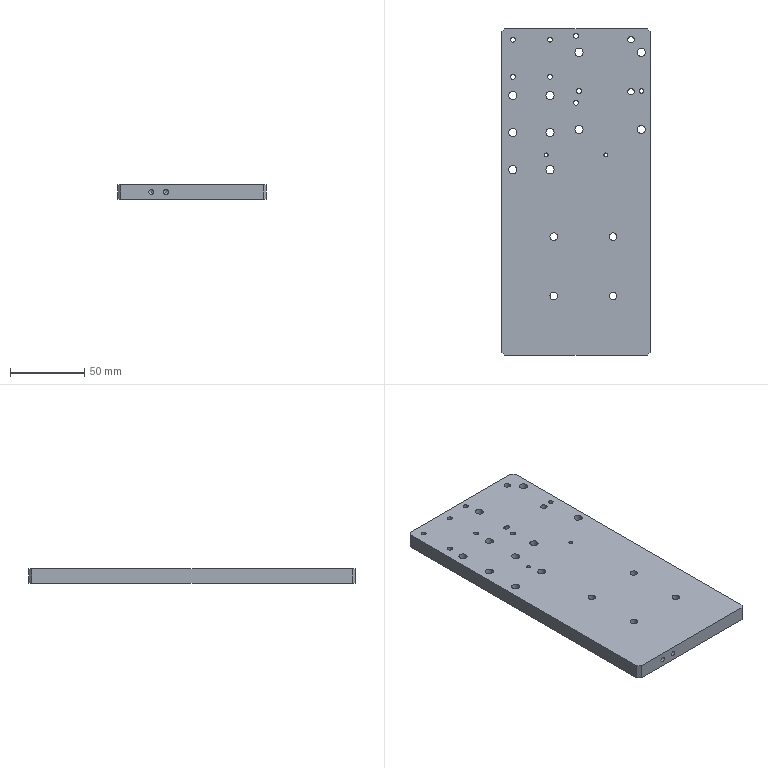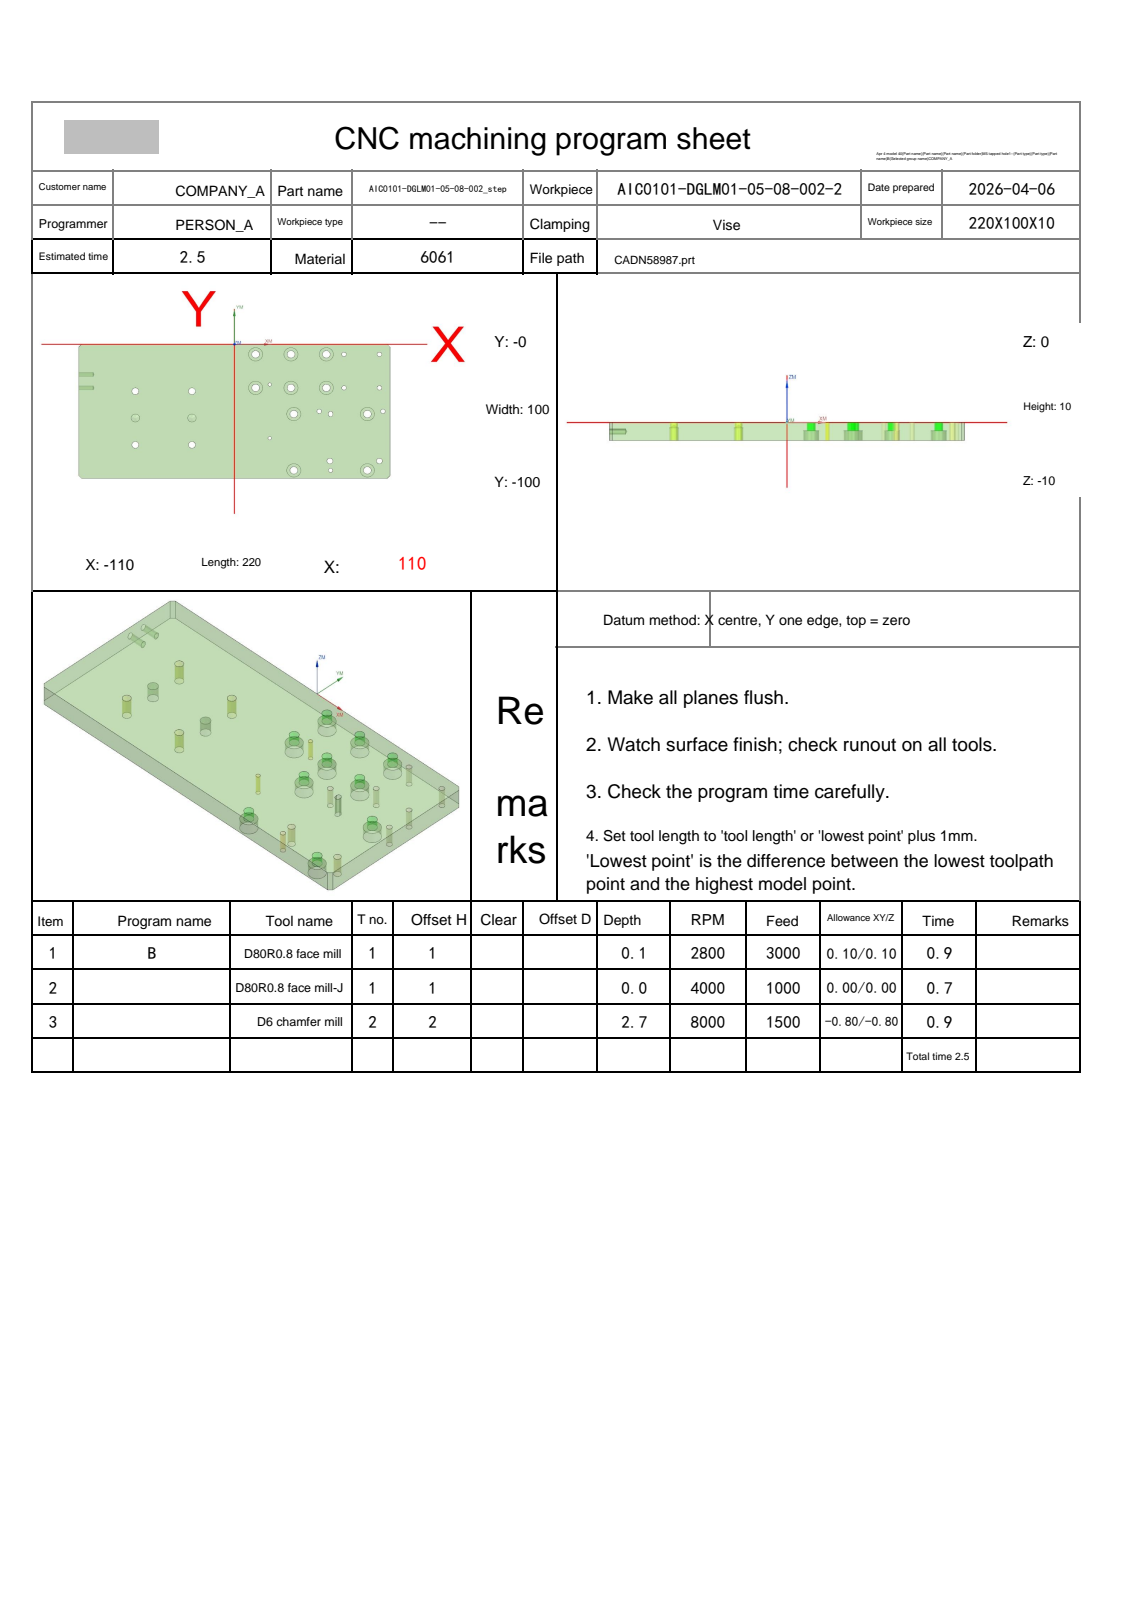NC program | NX | posted by the shop | part box 100 x 220 x 10 mm
Whole program:
%
O0001
(Machine time: 3.12 MIN)
(===Total Tool:2===)
(T1=D80R0.8 face mill D=80.  R=0.8  D-  H01 Z=-0.   )
(T2=D6 chamfer mill   D=6.   R=0.   D-  H02 Z=-2.7  )
G80 G90 G17 G49 G40
G91 G28 Z0
M01
N1 T01 M06
(D80R0.8 face mill  D=80. R=0.8 H=01 ce=0.10 di=0.10)
G00 G90 G54 X-162.097 Y-23.903 M03 S2800
G43 H01 Z20.
M08
Z3.525
G01 Z1.525 F3000.
X-150.097
X142.897
G02 X150.097 Y-31.103 I0.0 J-7.2
G01 Y-60.737
G02 X142.097 Y-68.737 I-8. J0.0
G01 X-150.097
X-162.097
Z3.525
G00 Y-23.903
Z3.05
G01 Z1.05
X-150.097
X142.897
G02 X150.097 Y-31.103 I0.0 J-7.2
G01 Y-60.737
G02 X142.097 Y-68.737 I-8. J0.0
G01 X-150.097
X-162.097
Z3.05
G00 Y-23.903
Z2.575
G01 Z.575
X-150.097
X142.897
G02 X150.097 Y-31.103 I0.0 J-7.2
G01 Y-60.737
G02 X142.097 Y-68.737 I-8. J0.0
G01 X-150.097
X-162.097
Z2.575
G00 Y-23.903
Z2.1
G01 Z.1
X-150.097
X142.897
G02 X150.097 Y-31.103 I0.0 J-7.2
G01 Y-60.737
G02 X142.097 Y-68.737 I-8. J0.0
G01 X-150.097
X-162.097
Z2.1
G00 Z20.
G91 G28 Z0.0
M05
M09
G91 G28 Z0.0
M01
N2 T01 M06
(D80R0.8 face mill-J  D=80. R=0.8 H=01 ce=0.00 di=0.00)
G00 G90 G54 X-161.999 Y-24.001 M03 S4000
G43 H01 Z20.
M08
Z2.
G01 Z0.0 F1000.
X-149.999
X142.799
G02 X149.999 Y-31.201 I0.0 J-7.2
G01 Y-60.639
G02 X141.999 Y-68.639 I-8. J0.0
G01 X-149.999
X-161.999
Z2.
G00 Z20.
G91 G28 Z0.0
M05
M09
G91 G28 Z0.0
M01
N3 T02 M06
(D6 chamfer mill  D=6. R=0. H=02 ce=0.00 di=0.00)
G00 G90 G54 X25. Y-30. M03 S8000
G43 H02 Z20.
M08
G98 G81 X25. Y-30. Z-1.75 R3. F1000.
Y-70.
G80
G00 Z20.
G00 G90 X68. Y-94. M03 S8000
Z20.
G98 G81 X68. Y-94. Z-1.8 R3. F1000.
G80
G00 Z20.
G00 G90 X105. Y-50. M03 S8000
Z20.
G98 G81 X105. Y-50. Z-2.2 R3. F1000.
X102.5 Y-32.5
Y-7.5
X77.5
Y-32.5
X60. Y-50.
G80
G00 Z20.
G00 G90 X67.5 Y-87. M03 S8000
Z20.
G98 G81 X67.5 Y-87. Z-2.7 R3. F1000.
X102.5
G80
G00 Z20.
G00 G90 X-30.87 Y-75.232 M03 S8000
Z20.
Z-.9
G01 Z-1.4 F600.
X-31.5 Y-75.4
G03 X-30. Y-76.9 I1.5 J0.0
X-28.1 Y-75. I0.0 J1.9
X-30. Y-73.1 I-1.9 J0.0
X-31.9 Y-75. I0.0 J-1.9
X-30. Y-76.9 I1.9 J0.0
X-28.5 Y-75.4 I0.0 J1.5
G01 X-29.13 Y-75.232
Z-.9
G00 Z20.
X-30.87 Y-35.232
Z-.9
G01 Z-1.4
X-31.5 Y-35.4
G03 X-30. Y-36.9 I1.5 J0.0
X-28.1 Y-35. I0.0 J1.9
X-30. Y-33.1 I-1.9 J0.0
X-31.9 Y-35. I0.0 J-1.9
X-30. Y-36.9 I1.9 J0.0
X-28.5 Y-35.4 I0.0 J1.5
G01 X-29.13 Y-35.232
Z-.9
G00 Z20.
X-70.87
Z-.9
G01 Z-1.4
X-71.5 Y-35.4
G03 X-70. Y-36.9 I1.5 J0.0
X-68.1 Y-35. I0.0 J1.9
X-70. Y-33.1 I-1.9 J0.0
X-71.9 Y-35. I0.0 J-1.9
X-70. Y-36.9 I1.9 J0.0
X-68.5 Y-35.4 I0.0 J1.5
G01 X-69.13 Y-35.232
Z-.9
G00 Z20.
X-70.87 Y-75.232
Z-.9
G01 Z-1.4
X-71.5 Y-75.4
G03 X-70. Y-76.9 I1.5 J0.0
X-68.1 Y-75. I0.0 J1.9
X-70. Y-73.1 I-1.9 J0.0
X-71.9 Y-75. I0.0 J-1.9
X-70. Y-76.9 I1.9 J0.0
X-68.5 Y-75.4 I0.0 J1.5
G01 X-69.13 Y-75.232
Z-.9
G00 Z20.
G00 G90 X93.353 Y-94.065 M03 S8000
Z20.
Z-.9
G01 Z-1.4 F1200.
X92.5 Y-94.15
G03 X94. Y-95.65 I1.5 J0.0
X95.65 Y-94. I0.0 J1.65
X94. Y-92.35 I-1.65 J0.0
X92.35 Y-94. I0.0 J-1.65
X94. Y-95.65 I1.65 J0.0
X95.5 Y-94.15 I0.0 J1.5
G01 X94.647 Y-94.065
Z-.9
G00 Z20.
X93.353 Y-52.065
Z-.9
G01 Z-1.4
X92.5 Y-52.15
G03 X94. Y-53.65 I1.5 J0.0
X95.65 Y-52. I0.0 J1.65
X94. Y-50.35 I-1.65 J0.0
X92.35 Y-52. I0.0 J-1.65
X94. Y-53.65 I1.65 J0.0
X95.5 Y-52.15 I0.0 J1.5
G01 X94.647 Y-52.065
Z-.9
G00 Z20.
X64.353 Y-32.565
Z-.9
G01 Z-1.4
X63.5 Y-32.65
G03 X65. Y-34.15 I1.5 J0.0
X66.65 Y-32.5 I0.0 J1.65
X65. Y-30.85 I-1.65 J0.0
X63.35 Y-32.5 I0.0 J-1.65
X65. Y-34.15 I1.65 J0.0
X66.5 Y-32.65 I0.0 J1.5
G01 X65.647 Y-32.565
Z-.9
G00 Z20.
X64.353 Y-7.565
Z-.9
G01 Z-1.4
X63.5 Y-7.65
G03 X65. Y-9.15 I1.5 J0.0
X66.65 Y-7.5 I0.0 J1.65
X65. Y-5.85 I-1.65 J0.0
X63.35 Y-7.5 I0.0 J-1.65
X65. Y-9.15 I1.65 J0.0
X66.5 Y-7.65 I0.0 J1.5
G01 X65.647 Y-7.565
Z-.9
G00 Z20.
X39.353
Z-.9
G01 Z-1.4
X38.5 Y-7.65
G03 X40. Y-9.15 I1.5 J0.0
X41.65 Y-7.5 I0.0 J1.65
X40. Y-5.85 I-1.65 J0.0
X38.35 Y-7.5 I0.0 J-1.65
X40. Y-9.15 I1.65 J0.0
X41.5 Y-7.65 I0.0 J1.5
G01 X40.647 Y-7.565
Z-.9
G00 Z20.
X14.353
Z-.9
G01 Z-1.4
X13.5 Y-7.65
G03 X15. Y-9.15 I1.5 J0.0
X16.65 Y-7.5 I0.0 J1.65
X15. Y-5.85 I-1.65 J0.0
X13.35 Y-7.5 I0.0 J-1.65
X15. Y-9.15 I1.65 J0.0
X16.5 Y-7.65 I0.0 J1.5
G01 X15.647 Y-7.565
Z-.9
G00 Z20.
X14.353 Y-32.565
Z-.9
G01 Z-1.4
X13.5 Y-32.65
G03 X15. Y-34.15 I1.5 J0.0
X16.65 Y-32.5 I0.0 J1.65
X15. Y-30.85 I-1.65 J0.0
X13.35 Y-32.5 I0.0 J-1.65
X15. Y-34.15 I1.65 J0.0
X16.5 Y-32.65 I0.0 J1.5
G01 X15.647 Y-32.565
Z-.9
G00 Z20.
X39.353
Z-.9
G01 Z-1.4
X38.5 Y-32.65
G03 X40. Y-34.15 I1.5 J0.0
X41.65 Y-32.5 I0.0 J1.65
X40. Y-30.85 I-1.65 J0.0
X38.35 Y-32.5 I0.0 J-1.65
X40. Y-34.15 I1.65 J0.0
X41.5 Y-32.65 I0.0 J1.5
G01 X40.647 Y-32.565
Z-.9
G00 Z20.
X41.353 Y-52.065
Z-.9
G01 Z-1.4
X40.5 Y-52.15
G03 X42. Y-53.65 I1.5 J0.0
X43.65 Y-52. I0.0 J1.65
X42. Y-50.35 I-1.65 J0.0
X40.35 Y-52. I0.0 J-1.65
X42. Y-53.65 I1.65 J0.0
X43.5 Y-52.15 I0.0 J1.5
G01 X42.647 Y-52.065
Z-.9
G00 Z20.
X41.353 Y-94.065
Z-.9
G01 Z-1.4
X40.5 Y-94.15
G03 X42. Y-95.65 I1.5 J0.0
X43.65 Y-94. I0.0 J1.65
X42. Y-92.35 I-1.65 J0.0
X40.35 Y-94. I0.0 J-1.65
X42. Y-95.65 I1.65 J0.0
X43.5 Y-94.15 I0.0 J1.5
G01 X42.647 Y-94.065
Z-.9
G00 Z20.
G00 G90 X-110.7 Y-10.954 M03 S7000
Z20.
Z2.5
G01 Y-2.124 Z-.714 F1500.
Y-2.047 Z-.742
X-110.662 Y-1.84 Z-.819
X-110.581 Y-1.645 Z-.895
X-110.462 Y-1.472 Z-.972
X-110.407 Y-1.417 Z-1.
X-108.583 Y.407
G02 X-107.876 Y.7 I.707 J-.707
G01 X107.876
G02 X108.583 Y.407 I0.0 J-1.
G01 X110.407 Y-1.417
G02 X110.7 Y-2.124 I-.707 J-.707
G01 Y-97.876
G02 X110.407 Y-98.583 I-1. J0.0
G01 X108.583 Y-100.407
G02 X107.876 Y-100.7 I-.707 J.707
G01 X-107.876
G02 X-108.583 Y-100.407 I0.0 J1.
G01 X-110.407 Y-98.583
G02 X-110.7 Y-97.876 I.707 J.707
G01 Y-2.124
G02 X-110.407 Y-1.417 I1. J0.0
G01 X-110.054 Y-1.064
Z1.5
G00 Z20.
X67.687 Y-53.234
Z2.5
G01 X67.748 Y-53.262 Z2.476
X67.931 Y-53.3 Z2.408
X68.069 Z2.357
X68.252 Y-53.262 Z2.289
X68.421 Y-53.184 Z2.221
X68.568 Y-53.068 Z2.153
X68.684 Y-52.921 Z2.085
X68.762 Y-52.752 Z2.018
X68.8 Y-52.569 Z1.95
Y-51.431 Z1.535
X68.762 Y-51.248 Z1.467
X68.684 Y-51.079 Z1.399
X68.568 Y-50.932 Z1.331
X68.421 Y-50.816 Z1.263
X68.252 Y-50.738 Z1.195
X68.069 Y-50.7 Z1.128
X67.931 Z1.077
X67.748 Y-50.738 Z1.009
X67.579 Y-50.816 Z.941
X67.432 Y-50.932 Z.873
X67.316 Y-51.079 Z.805
X67.238 Y-51.248 Z.737
X67.2 Y-51.431 Z.669
Y-52.569 Z.255
X67.238 Y-52.752 Z.187
X67.316 Y-52.921 Z.119
X67.432 Y-53.068 Z.051
X67.579 Y-53.184 Z-.017
X67.748 Y-53.262 Z-.085
X67.931 Y-53.3 Z-.153
X68.069 Z-.203
X68.252 Y-53.262 Z-.271
X68.421 Y-53.184 Z-.339
X68.568 Y-53.068 Z-.407
X68.684 Y-52.921 Z-.475
X68.762 Y-52.752 Z-.543
X68.8 Y-52.569 Z-.611
Y-51.5 Z-1.
G03 X68. Y-50.7 I-.8 J0.0
X67.2 Y-51.5 I0.0 J-.8
G01 Y-52.5
G03 X68. Y-53.3 I.8 J0.0
X68.8 Y-52.5 I0.0 J.8
G01 Y-51.5
G03 X68.649 Y-51.032 I-.8 J0.0
G01 Z1.5
G00 Z20.
M05
M09
G91 G28 Z0.0
G91 G28 Y0.0
M30
%